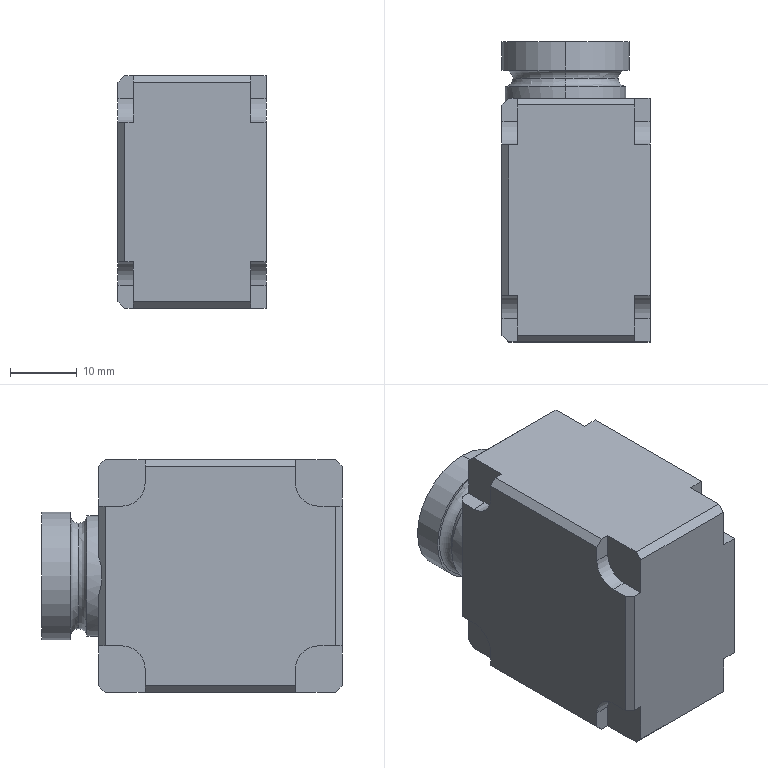Part | STEP file | 4-20.sldasm-Part-210 | 1 solid | 58 faces | box 22.225 x 45.05 x 34.95 mm | volume 29644 mm3 | plane 40 | cylinder 14 | torus 4 | commonest cylinder face diameters 7 x8 15.85 x2 18.1 x2 19.1 x2